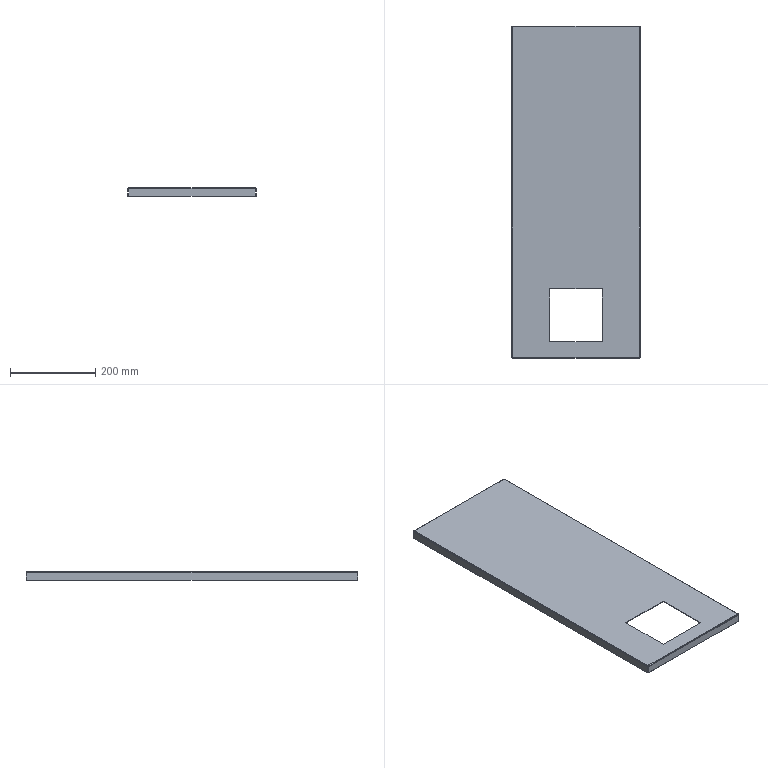Part | STEP file | X77-03011 | 1 solid | 42 faces | box 301 x 778 x 20 mm | volume 385520 mm3 | plane 26 | spline 8 | cylinder 8 | commonest cylinder face diameters 1.473 x4 4.473 x4